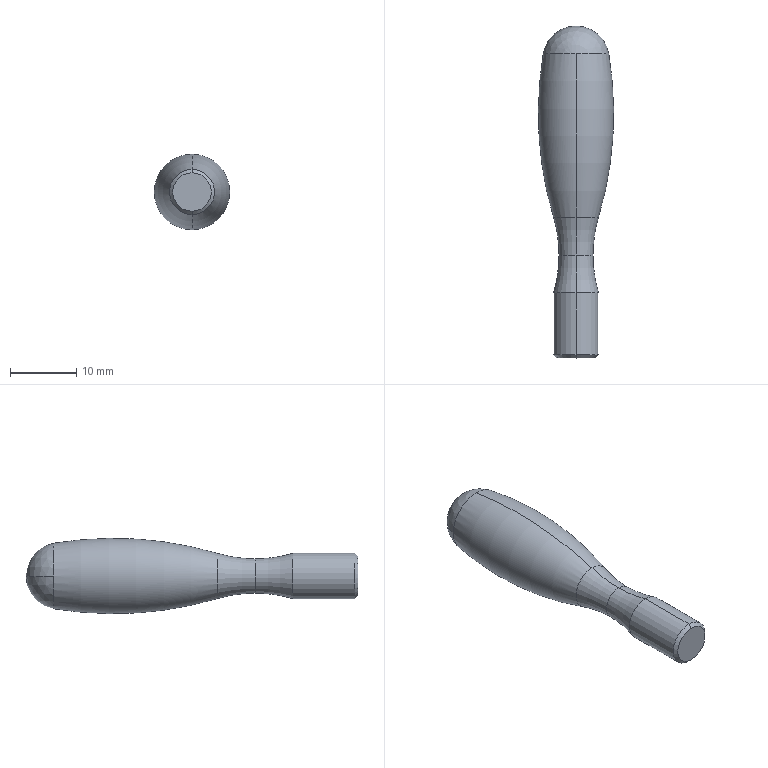Part | SolidWorks | features Revolution 1 | 1 solid | 13 faces | box 11.343 x 50 x 11.343 mm | volume 2889 mm3 | torus 6 | sphere 2 | cylinder 2 | cone 2 | plane 1 | commonest cylinder face diameters 6.8 x2
STEP:
#1=CARTESIAN_POINT('',(-106.5,97.077,-3.4));
#2=VERTEX_POINT('',#1);
#3=CARTESIAN_POINT('',(-106.5,102.765,-2.574));
#4=VERTEX_POINT('',#3);
#5=CARTESIAN_POINT('',(-106.5,102.765,-22.574));
#6=DIRECTION('',(-1.,0.,0.));
#7=DIRECTION('',(0.,0.,1.));
#8=AXIS2_PLACEMENT_3D('',#5,#6,#7);
#9=CIRCLE('',#8,20.);
#10=EDGE_CURVE('',#2,#4,#9,.T.);
#11=ORIENTED_EDGE('',*,*,#10,.T.);
#12=CARTESIAN_POINT('',(-106.5,102.765,2.574));
#13=VERTEX_POINT('',#12);
#14=CARTESIAN_POINT('',(-106.5,102.765,0.));
#15=DIRECTION('',(0.,-1.,0.));
#16=DIRECTION('',(0.,0.,-1.));
#17=AXIS2_PLACEMENT_3D('',#14,#15,#16);
#18=CIRCLE('',#17,2.574);
#19=EDGE_CURVE('',#4,#13,#18,.T.);
#20=ORIENTED_EDGE('',*,*,#19,.T.);
#21=CARTESIAN_POINT('',(-106.5,97.077,3.4));
#22=VERTEX_POINT('',#21);
#23=CARTESIAN_POINT('',(-106.5,102.765,22.574));
#24=DIRECTION('',(1.,0.,0.));
#25=DIRECTION('',(0.,0.,-1.));
#26=AXIS2_PLACEMENT_3D('',#23,#24,#25);
#27=CIRCLE('',#26,20.);
#28=EDGE_CURVE('',#22,#13,#27,.T.);
#29=ORIENTED_EDGE('',*,*,#28,.F.);
#30=CARTESIAN_POINT('',(-106.5,97.077,0.));
#31=DIRECTION('',(0.,-1.,0.));
#32=DIRECTION('',(0.,0.,-1.));
#33=AXIS2_PLACEMENT_3D('',#30,#31,#32);
#34=CIRCLE('',#33,3.4);
#35=EDGE_CURVE('',#2,#22,#34,.T.);
#36=ORIENTED_EDGE('',*,*,#35,.F.);
#37=EDGE_LOOP('',(#11,#20,#29,#36));
#38=FACE_OUTER_BOUND('',#37,.T.);
#39=CARTESIAN_POINT('',(-106.5,102.765,0.));
#40=DIRECTION('',(0.,-1.,0.));
#41=DIRECTION('',(0.,0.,-1.));
#42=AXIS2_PLACEMENT_3D('',#39,#40,#41);
#43=TOROIDAL_SURFACE('',#42,22.574,20.);
#44=ADVANCED_FACE('',(#38),#43,.F.);
#45=ORIENTED_EDGE('',*,*,#28,.T.);
#46=CARTESIAN_POINT('',(-106.5,102.765,0.));
#47=DIRECTION('',(0.,-1.,0.));
#48=DIRECTION('',(0.,0.,-1.));
#49=AXIS2_PLACEMENT_3D('',#46,#47,#48);
#50=CIRCLE('',#49,2.574);
#51=EDGE_CURVE('',#13,#4,#50,.T.);
#52=ORIENTED_EDGE('',*,*,#51,.T.);
#53=ORIENTED_EDGE('',*,*,#10,.F.);
#54=CARTESIAN_POINT('',(-106.5,97.077,0.));
#55=DIRECTION('',(0.,-1.,0.));
#56=DIRECTION('',(0.,0.,-1.));
#57=AXIS2_PLACEMENT_3D('',#54,#55,#56);
#58=CIRCLE('',#57,3.4);
#59=EDGE_CURVE('',#22,#2,#58,.T.);
#60=ORIENTED_EDGE('',*,*,#59,.F.);
#61=EDGE_LOOP('',(#45,#52,#53,#60));
#62=FACE_OUTER_BOUND('',#61,.T.);
#63=CARTESIAN_POINT('',(-106.5,102.765,0.));
#64=DIRECTION('',(0.,-1.,0.));
#65=DIRECTION('',(0.,0.,-1.));
#66=AXIS2_PLACEMENT_3D('',#63,#64,#65);
#67=TOROIDAL_SURFACE('',#66,22.574,20.);
#68=ADVANCED_FACE('',(#62),#67,.F.);
#69=ORIENTED_EDGE('',*,*,#35,.T.);
#70=CARTESIAN_POINT('',(-106.5,87.763,3.4));
#71=VERTEX_POINT('',#70);
#72=CARTESIAN_POINT('',(-106.5,85.3,3.4));
#73=DIRECTION('',(0.,-1.,0.));
#74=VECTOR('',#73,1000.);
#75=LINE('',#72,#74);
#76=EDGE_CURVE('',#22,#71,#75,.T.);
#77=ORIENTED_EDGE('',*,*,#76,.T.);
#78=CARTESIAN_POINT('',(-106.5,87.763,-3.4));
#79=VERTEX_POINT('',#78);
#80=CARTESIAN_POINT('',(-106.5,87.763,0.));
#81=DIRECTION('',(0.,-1.,0.));
#82=DIRECTION('',(0.,0.,-1.));
#83=AXIS2_PLACEMENT_3D('',#80,#81,#82);
#84=CIRCLE('',#83,3.4);
#85=EDGE_CURVE('',#79,#71,#84,.T.);
#86=ORIENTED_EDGE('',*,*,#85,.F.);
#87=CARTESIAN_POINT('',(-106.5,85.3,-3.4));
#88=DIRECTION('',(0.,-1.,0.));
#89=VECTOR('',#88,1000.);
#90=LINE('',#87,#89);
#91=EDGE_CURVE('',#2,#79,#90,.T.);
#92=ORIENTED_EDGE('',*,*,#91,.F.);
#93=EDGE_LOOP('',(#69,#77,#86,#92));
#94=FACE_OUTER_BOUND('',#93,.T.);
#95=CARTESIAN_POINT('',(-106.5,85.3,0.));
#96=DIRECTION('',(0.,-1.,0.));
#97=DIRECTION('',(0.,0.,-1.));
#98=AXIS2_PLACEMENT_3D('',#95,#96,#97);
#99=CYLINDRICAL_SURFACE('',#98,3.4);
#100=ADVANCED_FACE('',(#94),#99,.T.);
#101=CARTESIAN_POINT('',(-106.5,87.263,-2.9));
#102=VERTEX_POINT('',#101);
#103=CARTESIAN_POINT('',(-106.5,87.263,2.9));
#104=VERTEX_POINT('',#103);
#105=CARTESIAN_POINT('',(-106.5,87.263,0.));
#106=DIRECTION('',(0.,-1.,0.));
#107=DIRECTION('',(0.,0.,-1.));
#108=AXIS2_PLACEMENT_3D('',#105,#106,#107);
#109=CIRCLE('',#108,2.9);
#110=EDGE_CURVE('',#102,#104,#109,.T.);
#111=ORIENTED_EDGE('',*,*,#110,.F.);
#112=CARTESIAN_POINT('',(-106.5,87.263,-2.9));
#113=DIRECTION('',(0.,0.7071,-0.7071));
#114=VECTOR('',#113,1000.);
#115=LINE('',#112,#114);
#116=EDGE_CURVE('',#102,#79,#115,.T.);
#117=ORIENTED_EDGE('',*,*,#116,.T.);
#118=ORIENTED_EDGE('',*,*,#85,.T.);
#119=CARTESIAN_POINT('',(-106.5,87.263,2.9));
#120=DIRECTION('',(0.,0.7071,0.7071));
#121=VECTOR('',#120,1000.);
#122=LINE('',#119,#121);
#123=EDGE_CURVE('',#104,#71,#122,.T.);
#124=ORIENTED_EDGE('',*,*,#123,.F.);
#125=EDGE_LOOP('',(#111,#117,#118,#124));
#126=FACE_OUTER_BOUND('',#125,.T.);
#127=CARTESIAN_POINT('',(-106.5,87.263,0.));
#128=DIRECTION('',(0.,1.,0.));
#129=DIRECTION('',(0.,0.,1.));
#130=AXIS2_PLACEMENT_3D('',#127,#128,#129);
#131=CONICAL_SURFACE('',#130,2.9,0.7854);
#132=ADVANCED_FACE('',(#126),#131,.T.);
#133=CARTESIAN_POINT('',(-106.5,137.263,0.));
#134=VERTEX_POINT('',#133);
#135=CARTESIAN_POINT('',(-101.567,133.08,0.));
#136=VERTEX_POINT('',#135);
#137=CARTESIAN_POINT('',(-106.5,132.263,0.));
#138=DIRECTION('',(0.,0.,-1.));
#139=DIRECTION('',(-1.,0.,0.));
#140=AXIS2_PLACEMENT_3D('',#137,#138,#139);
#141=CIRCLE('',#140,5.);
#142=EDGE_CURVE('',#134,#136,#141,.T.);
#143=ORIENTED_EDGE('',*,*,#142,.F.);
#144=CARTESIAN_POINT('',(-111.433,133.08,0.));
#145=VERTEX_POINT('',#144);
#146=CARTESIAN_POINT('',(-106.5,132.263,0.));
#147=DIRECTION('',(0.,0.,1.));
#148=DIRECTION('',(1.,0.,0.));
#149=AXIS2_PLACEMENT_3D('',#146,#147,#148);
#150=CIRCLE('',#149,5.);
#151=EDGE_CURVE('',#134,#145,#150,.T.);
#152=ORIENTED_EDGE('',*,*,#151,.T.);
#153=CARTESIAN_POINT('',(-106.5,133.08,4.933));
#154=VERTEX_POINT('',#153);
#155=CARTESIAN_POINT('',(-106.5,133.08,0.));
#156=DIRECTION('',(0.,-1.,0.));
#157=DIRECTION('',(0.,0.,-1.));
#158=AXIS2_PLACEMENT_3D('',#155,#156,#157);
#159=CIRCLE('',#158,4.933);
#160=EDGE_CURVE('',#154,#145,#159,.T.);
#161=ORIENTED_EDGE('',*,*,#160,.F.);
#162=CARTESIAN_POINT('',(-106.5,133.08,0.));
#163=DIRECTION('',(0.,-1.,0.));
#164=DIRECTION('',(0.,0.,-1.));
#165=AXIS2_PLACEMENT_3D('',#162,#163,#164);
#166=CIRCLE('',#165,4.933);
#167=EDGE_CURVE('',#136,#154,#166,.T.);
#168=ORIENTED_EDGE('',*,*,#167,.F.);
#169=EDGE_LOOP('',(#143,#152,#161,#168));
#170=FACE_OUTER_BOUND('',#169,.T.);
#171=CARTESIAN_POINT('',(-106.5,132.263,0.));
#172=DIRECTION('',(0.,0.,1.));
#173=DIRECTION('',(1.,0.,0.));
#174=AXIS2_PLACEMENT_3D('',#171,#172,#173);
#175=SPHERICAL_SURFACE('',#174,5.);
#176=ADVANCED_FACE('',(#170),#175,.T.);
#177=CARTESIAN_POINT('',(-106.5,133.08,-4.933));
#178=VERTEX_POINT('',#177);
#179=CARTESIAN_POINT('',(-106.5,133.08,0.));
#180=DIRECTION('',(0.,-1.,0.));
#181=DIRECTION('',(0.,0.,-1.));
#182=AXIS2_PLACEMENT_3D('',#179,#180,#181);
#183=CIRCLE('',#182,4.933);
#184=EDGE_CURVE('',#178,#136,#183,.T.);
#185=ORIENTED_EDGE('',*,*,#184,.T.);
#186=ORIENTED_EDGE('',*,*,#167,.T.);
#187=CARTESIAN_POINT('',(-106.5,108.453,3.4));
#188=VERTEX_POINT('',#187);
#189=CARTESIAN_POINT('',(-106.5,124.096,-49.329));
#190=DIRECTION('',(1.,0.,0.));
#191=DIRECTION('',(0.,0.,-1.));
#192=AXIS2_PLACEMENT_3D('',#189,#190,#191);
#193=CIRCLE('',#192,55.);
#194=EDGE_CURVE('',#154,#188,#193,.T.);
#195=ORIENTED_EDGE('',*,*,#194,.T.);
#196=CARTESIAN_POINT('',(-106.5,108.453,-3.4));
#197=VERTEX_POINT('',#196);
#198=CARTESIAN_POINT('',(-106.5,108.453,0.));
#199=DIRECTION('',(0.,-1.,0.));
#200=DIRECTION('',(0.,0.,-1.));
#201=AXIS2_PLACEMENT_3D('',#198,#199,#200);
#202=CIRCLE('',#201,3.4);
#203=EDGE_CURVE('',#197,#188,#202,.T.);
#204=ORIENTED_EDGE('',*,*,#203,.F.);
#205=CARTESIAN_POINT('',(-106.5,124.096,49.329));
#206=DIRECTION('',(-1.,0.,0.));
#207=DIRECTION('',(0.,0.,1.));
#208=AXIS2_PLACEMENT_3D('',#205,#206,#207);
#209=CIRCLE('',#208,55.);
#210=EDGE_CURVE('',#178,#197,#209,.T.);
#211=ORIENTED_EDGE('',*,*,#210,.F.);
#212=EDGE_LOOP('',(#185,#186,#195,#204,#211));
#213=FACE_OUTER_BOUND('',#212,.T.);
#214=CARTESIAN_POINT('',(-106.5,124.096,0.));
#215=DIRECTION('',(0.,-1.,0.));
#216=DIRECTION('',(0.,0.,-1.));
#217=AXIS2_PLACEMENT_3D('',#214,#215,#216);
#218=TOROIDAL_SURFACE('',#217,-49.329,55.);
#219=ADVANCED_FACE('',(#213),#218,.T.);
#220=ORIENTED_EDGE('',*,*,#51,.F.);
#221=CARTESIAN_POINT('',(-106.5,102.765,22.574));
#222=DIRECTION('',(1.,0.,0.));
#223=DIRECTION('',(0.,0.,-1.));
#224=AXIS2_PLACEMENT_3D('',#221,#222,#223);
#225=CIRCLE('',#224,20.);
#226=EDGE_CURVE('',#13,#188,#225,.T.);
#227=ORIENTED_EDGE('',*,*,#226,.T.);
#228=CARTESIAN_POINT('',(-106.5,108.453,0.));
#229=DIRECTION('',(0.,-1.,0.));
#230=DIRECTION('',(0.,0.,-1.));
#231=AXIS2_PLACEMENT_3D('',#228,#229,#230);
#232=CIRCLE('',#231,3.4);
#233=EDGE_CURVE('',#188,#197,#232,.T.);
#234=ORIENTED_EDGE('',*,*,#233,.T.);
#235=CARTESIAN_POINT('',(-106.5,102.765,-22.574));
#236=DIRECTION('',(-1.,0.,0.));
#237=DIRECTION('',(0.,0.,1.));
#238=AXIS2_PLACEMENT_3D('',#235,#236,#237);
#239=CIRCLE('',#238,20.);
#240=EDGE_CURVE('',#4,#197,#239,.T.);
#241=ORIENTED_EDGE('',*,*,#240,.F.);
#242=EDGE_LOOP('',(#220,#227,#234,#241));
#243=FACE_OUTER_BOUND('',#242,.T.);
#244=CARTESIAN_POINT('',(-106.5,102.765,0.));
#245=DIRECTION('',(0.,-1.,0.));
#246=DIRECTION('',(0.,0.,-1.));
#247=AXIS2_PLACEMENT_3D('',#244,#245,#246);
#248=TOROIDAL_SURFACE('',#247,22.574,20.);
#249=ADVANCED_FACE('',(#243),#248,.F.);
#250=ORIENTED_EDGE('',*,*,#19,.F.);
#251=ORIENTED_EDGE('',*,*,#240,.T.);
#252=ORIENTED_EDGE('',*,*,#203,.T.);
#253=ORIENTED_EDGE('',*,*,#226,.F.);
#254=EDGE_LOOP('',(#250,#251,#252,#253));
#255=FACE_OUTER_BOUND('',#254,.T.);
#256=CARTESIAN_POINT('',(-106.5,102.765,0.));
#257=DIRECTION('',(0.,-1.,0.));
#258=DIRECTION('',(0.,0.,-1.));
#259=AXIS2_PLACEMENT_3D('',#256,#257,#258);
#260=TOROIDAL_SURFACE('',#259,22.574,20.);
#261=ADVANCED_FACE('',(#255),#260,.F.);
#262=ORIENTED_EDGE('',*,*,#194,.F.);
#263=ORIENTED_EDGE('',*,*,#160,.T.);
#264=CARTESIAN_POINT('',(-106.5,133.08,0.));
#265=DIRECTION('',(0.,-1.,0.));
#266=DIRECTION('',(0.,0.,-1.));
#267=AXIS2_PLACEMENT_3D('',#264,#265,#266);
#268=CIRCLE('',#267,4.933);
#269=EDGE_CURVE('',#145,#178,#268,.T.);
#270=ORIENTED_EDGE('',*,*,#269,.T.);
#271=ORIENTED_EDGE('',*,*,#210,.T.);
#272=ORIENTED_EDGE('',*,*,#233,.F.);
#273=EDGE_LOOP('',(#262,#263,#270,#271,#272));
#274=FACE_OUTER_BOUND('',#273,.T.);
#275=CARTESIAN_POINT('',(-106.5,124.096,0.));
#276=DIRECTION('',(0.,-1.,0.));
#277=DIRECTION('',(0.,0.,-1.));
#278=AXIS2_PLACEMENT_3D('',#275,#276,#277);
#279=TOROIDAL_SURFACE('',#278,-49.329,55.);
#280=ADVANCED_FACE('',(#274),#279,.T.);
#281=ORIENTED_EDGE('',*,*,#151,.F.);
#282=ORIENTED_EDGE('',*,*,#142,.T.);
#283=ORIENTED_EDGE('',*,*,#184,.F.);
#284=ORIENTED_EDGE('',*,*,#269,.F.);
#285=EDGE_LOOP('',(#281,#282,#283,#284));
#286=FACE_OUTER_BOUND('',#285,.T.);
#287=CARTESIAN_POINT('',(-106.5,132.263,0.));
#288=DIRECTION('',(0.,0.,1.));
#289=DIRECTION('',(1.,0.,0.));
#290=AXIS2_PLACEMENT_3D('',#287,#288,#289);
#291=SPHERICAL_SURFACE('',#290,5.);
#292=ADVANCED_FACE('',(#286),#291,.T.);
#293=CARTESIAN_POINT('',(-106.5,87.263,0.));
#294=DIRECTION('',(0.,-1.,0.));
#295=DIRECTION('',(0.,0.,-1.));
#296=AXIS2_PLACEMENT_3D('',#293,#294,#295);
#297=CIRCLE('',#296,2.9);
#298=EDGE_CURVE('',#104,#102,#297,.T.);
#299=ORIENTED_EDGE('',*,*,#298,.T.);
#300=ORIENTED_EDGE('',*,*,#110,.T.);
#301=EDGE_LOOP('',(#299,#300));
#302=FACE_OUTER_BOUND('',#301,.T.);
#303=CARTESIAN_POINT('',(-106.5,87.263,0.));
#304=DIRECTION('',(0.,-1.,0.));
#305=DIRECTION('',(0.,0.,-1.));
#306=AXIS2_PLACEMENT_3D('',#303,#304,#305);
#307=PLANE('',#306);
#308=ADVANCED_FACE('',(#302),#307,.T.);
#309=ORIENTED_EDGE('',*,*,#116,.F.);
#310=ORIENTED_EDGE('',*,*,#298,.F.);
#311=ORIENTED_EDGE('',*,*,#123,.T.);
#312=CARTESIAN_POINT('',(-106.5,87.763,0.));
#313=DIRECTION('',(0.,-1.,0.));
#314=DIRECTION('',(0.,0.,-1.));
#315=AXIS2_PLACEMENT_3D('',#312,#313,#314);
#316=CIRCLE('',#315,3.4);
#317=EDGE_CURVE('',#71,#79,#316,.T.);
#318=ORIENTED_EDGE('',*,*,#317,.T.);
#319=EDGE_LOOP('',(#309,#310,#311,#318));
#320=FACE_OUTER_BOUND('',#319,.T.);
#321=CARTESIAN_POINT('',(-106.5,87.263,0.));
#322=DIRECTION('',(0.,1.,0.));
#323=DIRECTION('',(0.,0.,1.));
#324=AXIS2_PLACEMENT_3D('',#321,#322,#323);
#325=CONICAL_SURFACE('',#324,2.9,0.7854);
#326=ADVANCED_FACE('',(#320),#325,.T.);
#327=ORIENTED_EDGE('',*,*,#76,.F.);
#328=ORIENTED_EDGE('',*,*,#59,.T.);
#329=ORIENTED_EDGE('',*,*,#91,.T.);
#330=ORIENTED_EDGE('',*,*,#317,.F.);
#331=EDGE_LOOP('',(#327,#328,#329,#330));
#332=FACE_OUTER_BOUND('',#331,.T.);
#333=CARTESIAN_POINT('',(-106.5,85.3,0.));
#334=DIRECTION('',(0.,-1.,0.));
#335=DIRECTION('',(0.,0.,-1.));
#336=AXIS2_PLACEMENT_3D('',#333,#334,#335);
#337=CYLINDRICAL_SURFACE('',#336,3.4);
#338=ADVANCED_FACE('',(#332),#337,.T.);
#339=CLOSED_SHELL('',(#44,#68,#100,#132,#176,#219,#249,#261,#280,#292,#308,#326,#338));
#340=MANIFOLD_SOLID_BREP('',#339);
#341=CARTESIAN_POINT('',(0.,0.,0.));
#342=DIRECTION('',(0.,0.,1.));
#343=DIRECTION('',(1.,0.,0.));
#344=AXIS2_PLACEMENT_3D('',#341,#342,#343);
#345=(LENGTH_UNIT()NAMED_UNIT(*)SI_UNIT(.MILLI.,.METRE.));
#346=UNCERTAINTY_MEASURE_WITH_UNIT(LENGTH_MEASURE(0.00001),#345,'','');
#347=(NAMED_UNIT(*)PLANE_ANGLE_UNIT()SI_UNIT($,.RADIAN.));
#348=(NAMED_UNIT(*)SI_UNIT($,.STERADIAN.)SOLID_ANGLE_UNIT());
#349=(GEOMETRIC_REPRESENTATION_CONTEXT(3)GLOBAL_UNCERTAINTY_ASSIGNED_CONTEXT((#346))GLOBAL_UNIT_ASSIGNED_CONTEXT((#345,#347,#348))REPRESENTATION_CONTEXT('',''));
#350=ADVANCED_BREP_SHAPE_REPRESENTATION('',(#340,#344),#349);